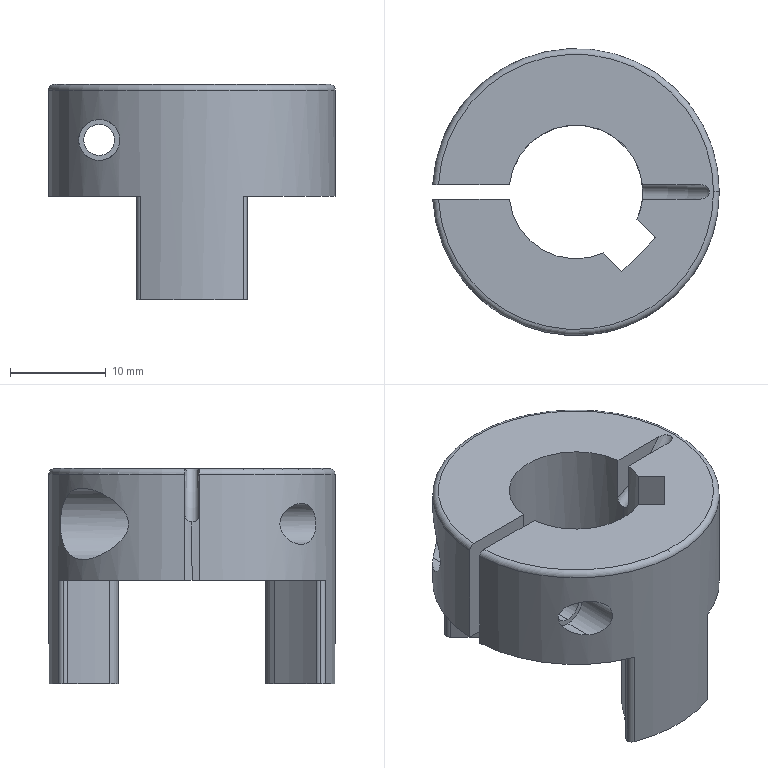Part | STEP file | BODY-L_E-LMPJC30L35-14-15-LK5 | 1 solid | 41 faces | box 29.981 x 30 x 22.5 mm | volume 6809 mm3 | cylinder 25 | plane 13 | torus 3 | commonest cylinder face diameters 1.2 x6 4.3 x4 61.94 x4 14 x3 3.242 x2 4.1 x2